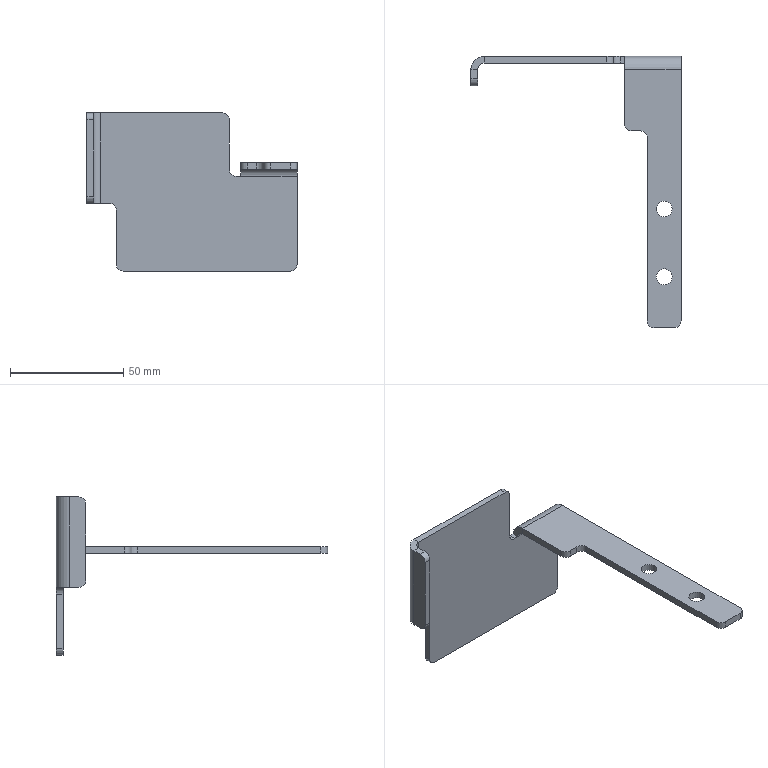Part | NX | features BREP 1 | 1 solid | 40 faces | box 93 x 120 x 70 mm | volume 23018 mm3 | plane 23 | cylinder 17 | commonest cylinder face diameters 6 x13 7 x2 12 x2
STEP:
#1=CARTESIAN_POINT('',(-17.5,-3.,-3.));
#2=VERTEX_POINT('',#1);
#3=CARTESIAN_POINT('',(-17.5,-3.,19.));
#4=VERTEX_POINT('',#3);
#5=CARTESIAN_POINT('',(-17.5,-3.,22.));
#6=DIRECTION('',(0.,0.,1.));
#7=VECTOR('',#6,1000.);
#8=LINE('',#5,#7);
#9=EDGE_CURVE('',#2,#4,#8,.T.);
#10=ORIENTED_EDGE('',*,*,#9,.T.);
#11=CARTESIAN_POINT('',(-20.5,-3.,22.));
#12=VERTEX_POINT('',#11);
#13=CARTESIAN_POINT('',(-20.5,-3.,19.));
#14=DIRECTION('',(0.,-1.,0.));
#15=DIRECTION('',(0.,0.,1.));
#16=AXIS2_PLACEMENT_3D('',#13,#14,#15);
#17=CIRCLE('',#16,3.);
#18=EDGE_CURVE('',#4,#12,#17,.T.);
#19=ORIENTED_EDGE('',*,*,#18,.T.);
#20=CARTESIAN_POINT('',(-74.5,-3.,22.));
#21=VERTEX_POINT('',#20);
#22=CARTESIAN_POINT('',(-77.5,-3.,22.));
#23=DIRECTION('',(-1.,0.,0.));
#24=VECTOR('',#23,1000.);
#25=LINE('',#22,#24);
#26=EDGE_CURVE('',#12,#21,#25,.T.);
#27=ORIENTED_EDGE('',*,*,#26,.T.);
#28=CARTESIAN_POINT('',(-74.5,-3.,-18.));
#29=VERTEX_POINT('',#28);
#30=CARTESIAN_POINT('',(-74.5,-3.,-48.));
#31=DIRECTION('',(0.,0.,1.));
#32=VECTOR('',#31,1000.);
#33=LINE('',#30,#32);
#34=EDGE_CURVE('',#29,#21,#33,.T.);
#35=ORIENTED_EDGE('',*,*,#34,.F.);
#36=CARTESIAN_POINT('',(-70.5,-3.,-18.));
#37=VERTEX_POINT('',#36);
#38=CARTESIAN_POINT('',(12.5,-3.,-18.));
#39=DIRECTION('',(1.,0.,0.));
#40=VECTOR('',#39,1000.);
#41=LINE('',#38,#40);
#42=EDGE_CURVE('',#29,#37,#41,.T.);
#43=ORIENTED_EDGE('',*,*,#42,.T.);
#44=CARTESIAN_POINT('',(-67.5,-3.,-21.));
#45=VERTEX_POINT('',#44);
#46=CARTESIAN_POINT('',(-70.5,-3.,-21.));
#47=DIRECTION('',(0.,1.,0.));
#48=DIRECTION('',(0.,0.,1.));
#49=AXIS2_PLACEMENT_3D('',#46,#47,#48);
#50=CIRCLE('',#49,3.);
#51=EDGE_CURVE('',#37,#45,#50,.T.);
#52=ORIENTED_EDGE('',*,*,#51,.T.);
#53=CARTESIAN_POINT('',(-67.5,-3.,-45.));
#54=VERTEX_POINT('',#53);
#55=CARTESIAN_POINT('',(-67.5,-3.,0.));
#56=DIRECTION('',(0.,0.,-1.));
#57=VECTOR('',#56,1000.);
#58=LINE('',#55,#57);
#59=EDGE_CURVE('',#45,#54,#58,.T.);
#60=ORIENTED_EDGE('',*,*,#59,.T.);
#61=CARTESIAN_POINT('',(-64.5,-3.,-48.));
#62=VERTEX_POINT('',#61);
#63=CARTESIAN_POINT('',(-64.5,-3.,-45.));
#64=DIRECTION('',(0.,-1.,0.));
#65=DIRECTION('',(0.,0.,1.));
#66=AXIS2_PLACEMENT_3D('',#63,#64,#65);
#67=CIRCLE('',#66,3.);
#68=EDGE_CURVE('',#54,#62,#67,.T.);
#69=ORIENTED_EDGE('',*,*,#68,.T.);
#70=CARTESIAN_POINT('',(9.5,-3.,-48.));
#71=VERTEX_POINT('',#70);
#72=CARTESIAN_POINT('',(12.5,-3.,-48.));
#73=DIRECTION('',(-1.,0.,0.));
#74=VECTOR('',#73,1000.);
#75=LINE('',#72,#74);
#76=EDGE_CURVE('',#71,#62,#75,.T.);
#77=ORIENTED_EDGE('',*,*,#76,.F.);
#78=CARTESIAN_POINT('',(12.5,-3.,-45.));
#79=VERTEX_POINT('',#78);
#80=CARTESIAN_POINT('',(9.5,-3.,-45.));
#81=DIRECTION('',(0.,-1.,0.));
#82=DIRECTION('',(0.,0.,1.));
#83=AXIS2_PLACEMENT_3D('',#80,#81,#82);
#84=CIRCLE('',#83,3.);
#85=EDGE_CURVE('',#71,#79,#84,.T.);
#86=ORIENTED_EDGE('',*,*,#85,.T.);
#87=CARTESIAN_POINT('',(12.5,-3.,-6.));
#88=VERTEX_POINT('',#87);
#89=CARTESIAN_POINT('',(12.5,-3.,0.));
#90=DIRECTION('',(0.,0.,-1.));
#91=VECTOR('',#90,1000.);
#92=LINE('',#89,#91);
#93=EDGE_CURVE('',#88,#79,#92,.T.);
#94=ORIENTED_EDGE('',*,*,#93,.F.);
#95=CARTESIAN_POINT('',(-12.5,-3.,-6.));
#96=VERTEX_POINT('',#95);
#97=CARTESIAN_POINT('',(12.5,-3.,-6.));
#98=DIRECTION('',(-1.,0.,0.));
#99=VECTOR('',#98,1000.);
#100=LINE('',#97,#99);
#101=EDGE_CURVE('',#88,#96,#100,.T.);
#102=ORIENTED_EDGE('',*,*,#101,.T.);
#103=CARTESIAN_POINT('',(-14.5,-3.,-6.));
#104=VERTEX_POINT('',#103);
#105=CARTESIAN_POINT('',(-17.5,-3.,-6.));
#106=DIRECTION('',(-1.,0.,0.));
#107=VECTOR('',#106,1000.);
#108=LINE('',#105,#107);
#109=EDGE_CURVE('',#96,#104,#108,.T.);
#110=ORIENTED_EDGE('',*,*,#109,.T.);
#111=CARTESIAN_POINT('',(-14.5,-3.,-3.));
#112=DIRECTION('',(0.,1.,0.));
#113=DIRECTION('',(0.,0.,1.));
#114=AXIS2_PLACEMENT_3D('',#111,#112,#113);
#115=CIRCLE('',#114,3.);
#116=EDGE_CURVE('',#104,#2,#115,.T.);
#117=ORIENTED_EDGE('',*,*,#116,.T.);
#118=EDGE_LOOP('',(#10,#19,#27,#35,#43,#52,#60,#69,#77,#86,#94,#102,#110,#117));
#119=FACE_BOUND('',#118,.T.);
#120=CARTESIAN_POINT('',(12.5,-3.,0.));
#121=DIRECTION('',(0.,1.,0.));
#122=DIRECTION('',(0.,0.,-1.));
#123=AXIS2_PLACEMENT_3D('',#120,#121,#122);
#124=PLANE('',#123);
#125=ADVANCED_FACE('',(#119),#124,.F.);
#126=CARTESIAN_POINT('',(9.5,0.,-48.));
#127=VERTEX_POINT('',#126);
#128=CARTESIAN_POINT('',(-64.5,0.,-48.));
#129=VERTEX_POINT('',#128);
#130=CARTESIAN_POINT('',(12.5,0.,-48.));
#131=DIRECTION('',(-1.,0.,0.));
#132=VECTOR('',#131,1000.);
#133=LINE('',#130,#132);
#134=EDGE_CURVE('',#127,#129,#133,.T.);
#135=ORIENTED_EDGE('',*,*,#134,.F.);
#136=CARTESIAN_POINT('',(9.5,0.,-48.));
#137=DIRECTION('',(0.,-1.,0.));
#138=VECTOR('',#137,1000.);
#139=LINE('',#136,#138);
#140=EDGE_CURVE('',#127,#71,#139,.T.);
#141=ORIENTED_EDGE('',*,*,#140,.T.);
#142=ORIENTED_EDGE('',*,*,#76,.T.);
#143=CARTESIAN_POINT('',(-64.5,0.,-48.));
#144=DIRECTION('',(0.,1.,0.));
#145=VECTOR('',#144,1000.);
#146=LINE('',#143,#145);
#147=EDGE_CURVE('',#62,#129,#146,.T.);
#148=ORIENTED_EDGE('',*,*,#147,.T.);
#149=EDGE_LOOP('',(#135,#141,#142,#148));
#150=FACE_BOUND('',#149,.T.);
#151=CARTESIAN_POINT('',(12.5,0.,-48.));
#152=DIRECTION('',(0.,0.,-1.));
#153=DIRECTION('',(1.,0.,0.));
#154=AXIS2_PLACEMENT_3D('',#151,#152,#153);
#155=PLANE('',#154);
#156=ADVANCED_FACE('',(#150),#155,.T.);
#157=CARTESIAN_POINT('',(-74.5,0.,22.));
#158=VERTEX_POINT('',#157);
#159=CARTESIAN_POINT('',(-20.5,0.,22.));
#160=VERTEX_POINT('',#159);
#161=CARTESIAN_POINT('',(-77.5,0.,22.));
#162=DIRECTION('',(1.,0.,0.));
#163=VECTOR('',#162,1000.);
#164=LINE('',#161,#163);
#165=EDGE_CURVE('',#158,#160,#164,.T.);
#166=ORIENTED_EDGE('',*,*,#165,.T.);
#167=CARTESIAN_POINT('',(-17.5,0.,19.));
#168=VERTEX_POINT('',#167);
#169=CARTESIAN_POINT('',(-20.5,0.,19.));
#170=DIRECTION('',(0.,1.,0.));
#171=DIRECTION('',(0.,0.,1.));
#172=AXIS2_PLACEMENT_3D('',#169,#170,#171);
#173=CIRCLE('',#172,3.);
#174=EDGE_CURVE('',#160,#168,#173,.T.);
#175=ORIENTED_EDGE('',*,*,#174,.T.);
#176=CARTESIAN_POINT('',(-17.5,0.,-3.));
#177=VERTEX_POINT('',#176);
#178=CARTESIAN_POINT('',(-17.5,0.,22.));
#179=DIRECTION('',(0.,0.,-1.));
#180=VECTOR('',#179,1000.);
#181=LINE('',#178,#180);
#182=EDGE_CURVE('',#168,#177,#181,.T.);
#183=ORIENTED_EDGE('',*,*,#182,.T.);
#184=CARTESIAN_POINT('',(-14.5,0.,-6.));
#185=VERTEX_POINT('',#184);
#186=CARTESIAN_POINT('',(-14.5,0.,-3.));
#187=DIRECTION('',(0.,-1.,0.));
#188=DIRECTION('',(0.,0.,1.));
#189=AXIS2_PLACEMENT_3D('',#186,#187,#188);
#190=CIRCLE('',#189,3.);
#191=EDGE_CURVE('',#177,#185,#190,.T.);
#192=ORIENTED_EDGE('',*,*,#191,.T.);
#193=CARTESIAN_POINT('',(-12.5,0.,-6.));
#194=VERTEX_POINT('',#193);
#195=CARTESIAN_POINT('',(-17.5,0.,-6.));
#196=DIRECTION('',(1.,0.,0.));
#197=VECTOR('',#196,1000.);
#198=LINE('',#195,#197);
#199=EDGE_CURVE('',#185,#194,#198,.T.);
#200=ORIENTED_EDGE('',*,*,#199,.T.);
#201=CARTESIAN_POINT('',(12.5,0.,-6.));
#202=VERTEX_POINT('',#201);
#203=CARTESIAN_POINT('',(12.5,0.,-6.));
#204=DIRECTION('',(-1.,0.,0.));
#205=VECTOR('',#204,1000.);
#206=LINE('',#203,#205);
#207=EDGE_CURVE('',#202,#194,#206,.T.);
#208=ORIENTED_EDGE('',*,*,#207,.F.);
#209=CARTESIAN_POINT('',(12.5,0.,-45.));
#210=VERTEX_POINT('',#209);
#211=CARTESIAN_POINT('',(12.5,0.,0.));
#212=DIRECTION('',(0.,0.,-1.));
#213=VECTOR('',#212,1000.);
#214=LINE('',#211,#213);
#215=EDGE_CURVE('',#202,#210,#214,.T.);
#216=ORIENTED_EDGE('',*,*,#215,.T.);
#217=CARTESIAN_POINT('',(9.5,0.,-45.));
#218=DIRECTION('',(0.,1.,0.));
#219=DIRECTION('',(0.,0.,1.));
#220=AXIS2_PLACEMENT_3D('',#217,#218,#219);
#221=CIRCLE('',#220,3.);
#222=EDGE_CURVE('',#210,#127,#221,.T.);
#223=ORIENTED_EDGE('',*,*,#222,.T.);
#224=ORIENTED_EDGE('',*,*,#134,.T.);
#225=CARTESIAN_POINT('',(-67.5,0.,-45.));
#226=VERTEX_POINT('',#225);
#227=CARTESIAN_POINT('',(-64.5,0.,-45.));
#228=DIRECTION('',(0.,1.,0.));
#229=DIRECTION('',(0.,0.,1.));
#230=AXIS2_PLACEMENT_3D('',#227,#228,#229);
#231=CIRCLE('',#230,3.);
#232=EDGE_CURVE('',#129,#226,#231,.T.);
#233=ORIENTED_EDGE('',*,*,#232,.T.);
#234=CARTESIAN_POINT('',(-67.5,0.,-21.));
#235=VERTEX_POINT('',#234);
#236=CARTESIAN_POINT('',(-67.5,0.,-48.));
#237=DIRECTION('',(0.,0.,-1.));
#238=VECTOR('',#237,1000.);
#239=LINE('',#236,#238);
#240=EDGE_CURVE('',#235,#226,#239,.T.);
#241=ORIENTED_EDGE('',*,*,#240,.F.);
#242=CARTESIAN_POINT('',(-70.5,0.,-18.));
#243=VERTEX_POINT('',#242);
#244=CARTESIAN_POINT('',(-70.5,0.,-21.));
#245=DIRECTION('',(0.,-1.,0.));
#246=DIRECTION('',(0.,0.,1.));
#247=AXIS2_PLACEMENT_3D('',#244,#245,#246);
#248=CIRCLE('',#247,3.);
#249=EDGE_CURVE('',#235,#243,#248,.T.);
#250=ORIENTED_EDGE('',*,*,#249,.T.);
#251=CARTESIAN_POINT('',(-74.5,0.,-18.));
#252=VERTEX_POINT('',#251);
#253=CARTESIAN_POINT('',(-67.5,0.,-18.));
#254=DIRECTION('',(1.,0.,0.));
#255=VECTOR('',#254,1000.);
#256=LINE('',#253,#255);
#257=EDGE_CURVE('',#252,#243,#256,.T.);
#258=ORIENTED_EDGE('',*,*,#257,.F.);
#259=CARTESIAN_POINT('',(-74.5,0.,-48.));
#260=DIRECTION('',(0.,0.,1.));
#261=VECTOR('',#260,1000.);
#262=LINE('',#259,#261);
#263=EDGE_CURVE('',#252,#158,#262,.T.);
#264=ORIENTED_EDGE('',*,*,#263,.T.);
#265=EDGE_LOOP('',(#166,#175,#183,#192,#200,#208,#216,#223,#224,#233,#241,#250,#258,#264));
#266=FACE_BOUND('',#265,.T.);
#267=CARTESIAN_POINT('',(12.5,0.,0.));
#268=DIRECTION('',(0.,1.,0.));
#269=DIRECTION('',(0.,0.,-1.));
#270=AXIS2_PLACEMENT_3D('',#267,#268,#269);
#271=PLANE('',#270);
#272=ADVANCED_FACE('',(#266),#271,.T.);
#273=CARTESIAN_POINT('',(12.5,0.,-6.));
#274=DIRECTION('',(0.,-1.,0.));
#275=VECTOR('',#274,1000.);
#276=LINE('',#273,#275);
#277=EDGE_CURVE('',#202,#88,#276,.T.);
#278=ORIENTED_EDGE('',*,*,#277,.F.);
#279=CARTESIAN_POINT('',(12.5,-6.,0.));
#280=VERTEX_POINT('',#279);
#281=CARTESIAN_POINT('',(12.5,-6.,-6.));
#282=DIRECTION('',(-1.,0.,0.));
#283=DIRECTION('',(0.,0.,-1.));
#284=AXIS2_PLACEMENT_3D('',#281,#282,#283);
#285=CIRCLE('',#284,6.);
#286=EDGE_CURVE('',#280,#202,#285,.T.);
#287=ORIENTED_EDGE('',*,*,#286,.F.);
#288=CARTESIAN_POINT('',(12.5,-6.,-3.));
#289=VERTEX_POINT('',#288);
#290=CARTESIAN_POINT('',(12.5,-6.,-3.));
#291=DIRECTION('',(0.,0.,1.));
#292=VECTOR('',#291,1000.);
#293=LINE('',#290,#292);
#294=EDGE_CURVE('',#289,#280,#293,.T.);
#295=ORIENTED_EDGE('',*,*,#294,.F.);
#296=CARTESIAN_POINT('',(12.5,-6.,-6.));
#297=DIRECTION('',(-1.,0.,0.));
#298=DIRECTION('',(0.,0.,-1.));
#299=AXIS2_PLACEMENT_3D('',#296,#297,#298);
#300=CIRCLE('',#299,3.);
#301=EDGE_CURVE('',#289,#88,#300,.T.);
#302=ORIENTED_EDGE('',*,*,#301,.T.);
#303=EDGE_LOOP('',(#278,#287,#295,#302));
#304=FACE_BOUND('',#303,.T.);
#305=CARTESIAN_POINT('',(12.5,0.,-6.));
#306=DIRECTION('',(1.,0.,0.));
#307=DIRECTION('',(0.,0.,1.));
#308=AXIS2_PLACEMENT_3D('',#305,#306,#307);
#309=PLANE('',#308);
#310=ADVANCED_FACE('',(#304),#309,.T.);
#311=ORIENTED_EDGE('',*,*,#93,.T.);
#312=CARTESIAN_POINT('',(12.5,-6.,-45.));
#313=DIRECTION('',(0.,1.,0.));
#314=VECTOR('',#313,1000.);
#315=LINE('',#312,#314);
#316=EDGE_CURVE('',#79,#210,#315,.T.);
#317=ORIENTED_EDGE('',*,*,#316,.T.);
#318=ORIENTED_EDGE('',*,*,#215,.F.);
#319=ORIENTED_EDGE('',*,*,#277,.T.);
#320=EDGE_LOOP('',(#311,#317,#318,#319));
#321=FACE_BOUND('',#320,.T.);
#322=CARTESIAN_POINT('',(12.5,-6.,-3.));
#323=DIRECTION('',(1.,0.,0.));
#324=DIRECTION('',(0.,0.,1.));
#325=AXIS2_PLACEMENT_3D('',#322,#323,#324);
#326=PLANE('',#325);
#327=ADVANCED_FACE('',(#321),#326,.T.);
#328=CARTESIAN_POINT('',(-12.5,-6.,0.));
#329=VERTEX_POINT('',#328);
#330=CARTESIAN_POINT('',(-12.5,-6.,-3.));
#331=VERTEX_POINT('',#330);
#332=CARTESIAN_POINT('',(-12.5,-6.,0.));
#333=DIRECTION('',(0.,0.,-1.));
#334=VECTOR('',#333,1000.);
#335=LINE('',#332,#334);
#336=EDGE_CURVE('',#329,#331,#335,.T.);
#337=ORIENTED_EDGE('',*,*,#336,.F.);
#338=CARTESIAN_POINT('',(-12.5,-6.,-6.));
#339=DIRECTION('',(-1.,0.,0.));
#340=DIRECTION('',(0.,0.,-1.));
#341=AXIS2_PLACEMENT_3D('',#338,#339,#340);
#342=CIRCLE('',#341,6.);
#343=EDGE_CURVE('',#329,#194,#342,.T.);
#344=ORIENTED_EDGE('',*,*,#343,.T.);
#345=CARTESIAN_POINT('',(-12.5,-3.,-6.));
#346=DIRECTION('',(0.,1.,0.));
#347=VECTOR('',#346,1000.);
#348=LINE('',#345,#347);
#349=EDGE_CURVE('',#96,#194,#348,.T.);
#350=ORIENTED_EDGE('',*,*,#349,.F.);
#351=CARTESIAN_POINT('',(-12.5,-6.,-6.));
#352=DIRECTION('',(-1.,0.,0.));
#353=DIRECTION('',(0.,0.,-1.));
#354=AXIS2_PLACEMENT_3D('',#351,#352,#353);
#355=CIRCLE('',#354,3.);
#356=EDGE_CURVE('',#331,#96,#355,.T.);
#357=ORIENTED_EDGE('',*,*,#356,.F.);
#358=EDGE_LOOP('',(#337,#344,#350,#357));
#359=FACE_BOUND('',#358,.T.);
#360=CARTESIAN_POINT('',(-12.5,-6.,0.));
#361=DIRECTION('',(-1.,0.,0.));
#362=DIRECTION('',(0.,0.,-1.));
#363=AXIS2_PLACEMENT_3D('',#360,#361,#362);
#364=PLANE('',#363);
#365=ADVANCED_FACE('',(#359),#364,.T.);
#366=CARTESIAN_POINT('',(-12.5,-30.,-3.));
#367=VERTEX_POINT('',#366);
#368=CARTESIAN_POINT('',(-12.5,-120.,-3.));
#369=DIRECTION('',(0.,1.,0.));
#370=VECTOR('',#369,1000.);
#371=LINE('',#368,#370);
#372=EDGE_CURVE('',#367,#331,#371,.T.);
#373=ORIENTED_EDGE('',*,*,#372,.F.);
#374=CARTESIAN_POINT('',(-12.5,-30.,0.));
#375=VERTEX_POINT('',#374);
#376=CARTESIAN_POINT('',(-12.5,-30.,0.));
#377=DIRECTION('',(0.,0.,1.));
#378=VECTOR('',#377,1000.);
#379=LINE('',#376,#378);
#380=EDGE_CURVE('',#367,#375,#379,.T.);
#381=ORIENTED_EDGE('',*,*,#380,.T.);
#382=CARTESIAN_POINT('',(-12.5,-120.,0.));
#383=DIRECTION('',(0.,1.,0.));
#384=VECTOR('',#383,1000.);
#385=LINE('',#382,#384);
#386=EDGE_CURVE('',#375,#329,#385,.T.);
#387=ORIENTED_EDGE('',*,*,#386,.T.);
#388=ORIENTED_EDGE('',*,*,#336,.T.);
#389=EDGE_LOOP('',(#373,#381,#387,#388));
#390=FACE_BOUND('',#389,.T.);
#391=CARTESIAN_POINT('',(-12.5,-3.,-6.));
#392=DIRECTION('',(-1.,0.,0.));
#393=DIRECTION('',(0.,0.,-1.));
#394=AXIS2_PLACEMENT_3D('',#391,#392,#393);
#395=PLANE('',#394);
#396=ADVANCED_FACE('',(#390),#395,.T.);
#397=ORIENTED_EDGE('',*,*,#343,.F.);
#398=CARTESIAN_POINT('',(12.5,-6.,0.));
#399=DIRECTION('',(-1.,0.,0.));
#400=VECTOR('',#399,1000.);
#401=LINE('',#398,#400);
#402=EDGE_CURVE('',#280,#329,#401,.T.);
#403=ORIENTED_EDGE('',*,*,#402,.F.);
#404=ORIENTED_EDGE('',*,*,#286,.T.);
#405=ORIENTED_EDGE('',*,*,#207,.T.);
#406=EDGE_LOOP('',(#397,#403,#404,#405));
#407=FACE_BOUND('',#406,.T.);
#408=CARTESIAN_POINT('',(12.5,-6.,-6.));
#409=DIRECTION('',(-1.,0.,0.));
#410=DIRECTION('',(0.,0.,-1.));
#411=AXIS2_PLACEMENT_3D('',#408,#409,#410);
#412=CYLINDRICAL_SURFACE('',#411,6.);
#413=ADVANCED_FACE('',(#407),#412,.T.);
#414=CARTESIAN_POINT('',(8.5,-67.5,0.));
#415=VERTEX_POINT('',#414);
#416=CARTESIAN_POINT('',(5.,-67.5,0.));
#417=DIRECTION('',(0.,0.,1.));
#418=DIRECTION('',(1.,0.,0.));
#419=AXIS2_PLACEMENT_3D('',#416,#417,#418);
#420=CIRCLE('',#419,3.5);
#421=EDGE_CURVE('',#415,#415,#420,.T.);
#422=ORIENTED_EDGE('',*,*,#421,.F.);
#423=EDGE_LOOP('',(#422));
#424=FACE_BOUND('',#423,.T.);
#425=CARTESIAN_POINT('',(8.5,-97.5,0.));
#426=VERTEX_POINT('',#425);
#427=CARTESIAN_POINT('',(5.,-97.5,0.));
#428=DIRECTION('',(0.,0.,1.));
#429=DIRECTION('',(1.,0.,0.));
#430=AXIS2_PLACEMENT_3D('',#427,#428,#429);
#431=CIRCLE('',#430,3.5);
#432=EDGE_CURVE('',#426,#426,#431,.T.);
#433=ORIENTED_EDGE('',*,*,#432,.F.);
#434=EDGE_LOOP('',(#433));
#435=FACE_BOUND('',#434,.T.);
#436=CARTESIAN_POINT('',(9.5,-120.,0.));
#437=VERTEX_POINT('',#436);
#438=CARTESIAN_POINT('',(0.5,-120.,0.));
#439=VERTEX_POINT('',#438);
#440=CARTESIAN_POINT('',(12.5,-120.,0.));
#441=DIRECTION('',(-1.,0.,0.));
#442=VECTOR('',#441,1000.);
#443=LINE('',#440,#442);
#444=EDGE_CURVE('',#437,#439,#443,.T.);
#445=ORIENTED_EDGE('',*,*,#444,.F.);
#446=CARTESIAN_POINT('',(12.5,-117.,0.));
#447=VERTEX_POINT('',#446);
#448=CARTESIAN_POINT('',(9.5,-117.,0.));
#449=DIRECTION('',(0.,0.,1.));
#450=DIRECTION('',(1.,0.,0.));
#451=AXIS2_PLACEMENT_3D('',#448,#449,#450);
#452=CIRCLE('',#451,3.);
#453=EDGE_CURVE('',#437,#447,#452,.T.);
#454=ORIENTED_EDGE('',*,*,#453,.T.);
#455=CARTESIAN_POINT('',(12.5,-120.,0.));
#456=DIRECTION('',(0.,1.,0.));
#457=VECTOR('',#456,1000.);
#458=LINE('',#455,#457);
#459=EDGE_CURVE('',#447,#280,#458,.T.);
#460=ORIENTED_EDGE('',*,*,#459,.T.);
#461=ORIENTED_EDGE('',*,*,#402,.T.);
#462=ORIENTED_EDGE('',*,*,#386,.F.);
#463=CARTESIAN_POINT('',(-9.5,-33.,0.));
#464=VERTEX_POINT('',#463);
#465=CARTESIAN_POINT('',(-9.5,-30.,0.));
#466=DIRECTION('',(0.,0.,1.));
#467=DIRECTION('',(1.,0.,0.));
#468=AXIS2_PLACEMENT_3D('',#465,#466,#467);
#469=CIRCLE('',#468,3.);
#470=EDGE_CURVE('',#375,#464,#469,.T.);
#471=ORIENTED_EDGE('',*,*,#470,.T.);
#472=CARTESIAN_POINT('',(-5.5,-33.,0.));
#473=VERTEX_POINT('',#472);
#474=CARTESIAN_POINT('',(-12.5,-33.,0.));
#475=DIRECTION('',(-1.,0.,0.));
#476=VECTOR('',#475,1000.);
#477=LINE('',#474,#476);
#478=EDGE_CURVE('',#473,#464,#477,.T.);
#479=ORIENTED_EDGE('',*,*,#478,.F.);
#480=CARTESIAN_POINT('',(-2.5,-36.,0.));
#481=VERTEX_POINT('',#480);
#482=CARTESIAN_POINT('',(-5.5,-36.,0.));
#483=DIRECTION('',(0.,0.,-1.));
#484=DIRECTION('',(1.,0.,0.));
#485=AXIS2_PLACEMENT_3D('',#482,#483,#484);
#486=CIRCLE('',#485,3.);
#487=EDGE_CURVE('',#473,#481,#486,.T.);
#488=ORIENTED_EDGE('',*,*,#487,.T.);
#489=CARTESIAN_POINT('',(-2.5,-117.,0.));
#490=VERTEX_POINT('',#489);
#491=CARTESIAN_POINT('',(-2.5,-120.,0.));
#492=DIRECTION('',(0.,1.,0.));
#493=VECTOR('',#492,1000.);
#494=LINE('',#491,#493);
#495=EDGE_CURVE('',#490,#481,#494,.T.);
#496=ORIENTED_EDGE('',*,*,#495,.F.);
#497=CARTESIAN_POINT('',(0.5,-117.,0.));
#498=DIRECTION('',(0.,0.,1.));
#499=DIRECTION('',(1.,0.,0.));
#500=AXIS2_PLACEMENT_3D('',#497,#498,#499);
#501=CIRCLE('',#500,3.);
#502=EDGE_CURVE('',#490,#439,#501,.T.);
#503=ORIENTED_EDGE('',*,*,#502,.T.);
#504=EDGE_LOOP('',(#445,#454,#460,#461,#462,#471,#479,#488,#496,#503));
#505=FACE_BOUND('',#504,.T.);
#506=CARTESIAN_POINT('',(12.5,-120.,0.));
#507=DIRECTION('',(0.,0.,1.));
#508=DIRECTION('',(-1.,0.,0.));
#509=AXIS2_PLACEMENT_3D('',#506,#507,#508);
#510=PLANE('',#509);
#511=ADVANCED_FACE('',(#424,#435,#505),#510,.T.);
#512=CARTESIAN_POINT('',(9.5,-120.,-3.));
#513=VERTEX_POINT('',#512);
#514=CARTESIAN_POINT('',(0.5,-120.,-3.));
#515=VERTEX_POINT('',#514);
#516=CARTESIAN_POINT('',(12.5,-120.,-3.));
#517=DIRECTION('',(-1.,0.,0.));
#518=VECTOR('',#517,1000.);
#519=LINE('',#516,#518);
#520=EDGE_CURVE('',#513,#515,#519,.T.);
#521=ORIENTED_EDGE('',*,*,#520,.F.);
#522=CARTESIAN_POINT('',(9.5,-120.,-3.));
#523=DIRECTION('',(0.,0.,1.));
#524=VECTOR('',#523,1000.);
#525=LINE('',#522,#524);
#526=EDGE_CURVE('',#513,#437,#525,.T.);
#527=ORIENTED_EDGE('',*,*,#526,.T.);
#528=ORIENTED_EDGE('',*,*,#444,.T.);
#529=CARTESIAN_POINT('',(0.5,-120.,-3.));
#530=DIRECTION('',(0.,0.,-1.));
#531=VECTOR('',#530,1000.);
#532=LINE('',#529,#531);
#533=EDGE_CURVE('',#439,#515,#532,.T.);
#534=ORIENTED_EDGE('',*,*,#533,.T.);
#535=EDGE_LOOP('',(#521,#527,#528,#534));
#536=FACE_BOUND('',#535,.T.);
#537=CARTESIAN_POINT('',(12.5,-120.,-3.));
#538=DIRECTION('',(0.,-1.,0.));
#539=DIRECTION('',(0.,0.,1.));
#540=AXIS2_PLACEMENT_3D('',#537,#538,#539);
#541=PLANE('',#540);
#542=ADVANCED_FACE('',(#536),#541,.T.);
#543=CARTESIAN_POINT('',(8.5,-67.5,-3.));
#544=VERTEX_POINT('',#543);
#545=CARTESIAN_POINT('',(5.,-67.5,-3.));
#546=DIRECTION('',(0.,0.,1.));
#547=DIRECTION('',(1.,0.,0.));
#548=AXIS2_PLACEMENT_3D('',#545,#546,#547);
#549=CIRCLE('',#548,3.5);
#550=EDGE_CURVE('',#544,#544,#549,.T.);
#551=ORIENTED_EDGE('',*,*,#550,.T.);
#552=EDGE_LOOP('',(#551));
#553=FACE_BOUND('',#552,.T.);
#554=CARTESIAN_POINT('',(8.5,-97.5,-3.));
#555=VERTEX_POINT('',#554);
#556=CARTESIAN_POINT('',(5.,-97.5,-3.));
#557=DIRECTION('',(0.,0.,1.));
#558=DIRECTION('',(1.,0.,0.));
#559=AXIS2_PLACEMENT_3D('',#556,#557,#558);
#560=CIRCLE('',#559,3.5);
#561=EDGE_CURVE('',#555,#555,#560,.T.);
#562=ORIENTED_EDGE('',*,*,#561,.T.);
#563=EDGE_LOOP('',(#562));
#564=FACE_BOUND('',#563,.T.);
#565=CARTESIAN_POINT('',(12.5,-117.,-3.));
#566=VERTEX_POINT('',#565);
#567=CARTESIAN_POINT('',(12.5,-120.,-3.));
#568=DIRECTION('',(0.,1.,0.));
#569=VECTOR('',#568,1000.);
#570=LINE('',#567,#569);
#571=EDGE_CURVE('',#566,#289,#570,.T.);
#572=ORIENTED_EDGE('',*,*,#571,.F.);
#573=CARTESIAN_POINT('',(9.5,-117.,-3.));
#574=DIRECTION('',(0.,0.,-1.));
#575=DIRECTION('',(1.,0.,0.));
#576=AXIS2_PLACEMENT_3D('',#573,#574,#575);
#577=CIRCLE('',#576,3.);
#578=EDGE_CURVE('',#566,#513,#577,.T.);
#579=ORIENTED_EDGE('',*,*,#578,.T.);
#580=ORIENTED_EDGE('',*,*,#520,.T.);
#581=CARTESIAN_POINT('',(-2.5,-117.,-3.));
#582=VERTEX_POINT('',#581);
#583=CARTESIAN_POINT('',(0.5,-117.,-3.));
#584=DIRECTION('',(0.,0.,-1.));
#585=DIRECTION('',(1.,0.,0.));
#586=AXIS2_PLACEMENT_3D('',#583,#584,#585);
#587=CIRCLE('',#586,3.);
#588=EDGE_CURVE('',#515,#582,#587,.T.);
#589=ORIENTED_EDGE('',*,*,#588,.T.);
#590=CARTESIAN_POINT('',(-2.5,-36.,-3.));
#591=VERTEX_POINT('',#590);
#592=CARTESIAN_POINT('',(-2.5,-120.,-3.));
#593=DIRECTION('',(0.,-1.,0.));
#594=VECTOR('',#593,1000.);
#595=LINE('',#592,#594);
#596=EDGE_CURVE('',#591,#582,#595,.T.);
#597=ORIENTED_EDGE('',*,*,#596,.F.);
#598=CARTESIAN_POINT('',(-5.5,-33.,-3.));
#599=VERTEX_POINT('',#598);
#600=CARTESIAN_POINT('',(-5.5,-36.,-3.));
#601=DIRECTION('',(0.,0.,1.));
#602=DIRECTION('',(1.,0.,0.));
#603=AXIS2_PLACEMENT_3D('',#600,#601,#602);
#604=CIRCLE('',#603,3.);
#605=EDGE_CURVE('',#591,#599,#604,.T.);
#606=ORIENTED_EDGE('',*,*,#605,.T.);
#607=CARTESIAN_POINT('',(-9.5,-33.,-3.));
#608=VERTEX_POINT('',#607);
#609=CARTESIAN_POINT('',(-12.5,-33.,-3.));
#610=DIRECTION('',(1.,0.,0.));
#611=VECTOR('',#610,1000.);
#612=LINE('',#609,#611);
#613=EDGE_CURVE('',#608,#599,#612,.T.);
#614=ORIENTED_EDGE('',*,*,#613,.F.);
#615=CARTESIAN_POINT('',(-9.5,-30.,-3.));
#616=DIRECTION('',(0.,0.,-1.));
#617=DIRECTION('',(1.,0.,0.));
#618=AXIS2_PLACEMENT_3D('',#615,#616,#617);
#619=CIRCLE('',#618,3.);
#620=EDGE_CURVE('',#608,#367,#619,.T.);
#621=ORIENTED_EDGE('',*,*,#620,.T.);
#622=ORIENTED_EDGE('',*,*,#372,.T.);
#623=CARTESIAN_POINT('',(12.5,-6.,-3.));
#624=DIRECTION('',(-1.,0.,0.));
#625=VECTOR('',#624,1000.);
#626=LINE('',#623,#625);
#627=EDGE_CURVE('',#289,#331,#626,.T.);
#628=ORIENTED_EDGE('',*,*,#627,.F.);
#629=EDGE_LOOP('',(#572,#579,#580,#589,#597,#606,#614,#621,#622,#628));
#630=FACE_BOUND('',#629,.T.);
#631=CARTESIAN_POINT('',(12.5,-120.,-3.));
#632=DIRECTION('',(0.,0.,1.));
#633=DIRECTION('',(-1.,0.,0.));
#634=AXIS2_PLACEMENT_3D('',#631,#632,#633);
#635=PLANE('',#634);
#636=ADVANCED_FACE('',(#553,#564,#630),#635,.F.);
#637=ORIENTED_EDGE('',*,*,#356,.T.);
#638=ORIENTED_EDGE('',*,*,#101,.F.);
#639=ORIENTED_EDGE('',*,*,#301,.F.);
#640=ORIENTED_EDGE('',*,*,#627,.T.);
#641=EDGE_LOOP('',(#637,#638,#639,#640));
#642=FACE_BOUND('',#641,.T.);
#643=CARTESIAN_POINT('',(12.5,-6.,-6.));
#644=DIRECTION('',(-1.,0.,0.));
#645=DIRECTION('',(0.,0.,-1.));
#646=AXIS2_PLACEMENT_3D('',#643,#644,#645);
#647=CYLINDRICAL_SURFACE('',#646,3.);
#648=ADVANCED_FACE('',(#642),#647,.F.);
#649=ORIENTED_EDGE('',*,*,#459,.F.);
#650=CARTESIAN_POINT('',(12.5,-117.,-6.));
#651=DIRECTION('',(0.,0.,-1.));
#652=VECTOR('',#651,1000.);
#653=LINE('',#650,#652);
#654=EDGE_CURVE('',#447,#566,#653,.T.);
#655=ORIENTED_EDGE('',*,*,#654,.T.);
#656=ORIENTED_EDGE('',*,*,#571,.T.);
#657=ORIENTED_EDGE('',*,*,#294,.T.);
#658=EDGE_LOOP('',(#649,#655,#656,#657));
#659=FACE_BOUND('',#658,.T.);
#660=CARTESIAN_POINT('',(12.5,-6.,-6.));
#661=DIRECTION('',(1.,0.,0.));
#662=DIRECTION('',(0.,0.,1.));
#663=AXIS2_PLACEMENT_3D('',#660,#661,#662);
#664=PLANE('',#663);
#665=ADVANCED_FACE('',(#659),#664,.T.);
#666=ORIENTED_EDGE('',*,*,#199,.F.);
#667=CARTESIAN_POINT('',(-14.5,-3.,-6.));
#668=DIRECTION('',(0.,-1.,0.));
#669=VECTOR('',#668,1000.);
#670=LINE('',#667,#669);
#671=EDGE_CURVE('',#185,#104,#670,.T.);
#672=ORIENTED_EDGE('',*,*,#671,.T.);
#673=ORIENTED_EDGE('',*,*,#109,.F.);
#674=ORIENTED_EDGE('',*,*,#349,.T.);
#675=EDGE_LOOP('',(#666,#672,#673,#674));
#676=FACE_BOUND('',#675,.T.);
#677=CARTESIAN_POINT('',(-17.5,-98.525,-6.));
#678=DIRECTION('',(0.,0.,1.));
#679=DIRECTION('',(-1.,0.,0.));
#680=AXIS2_PLACEMENT_3D('',#677,#678,#679);
#681=PLANE('',#680);
#682=ADVANCED_FACE('',(#676),#681,.T.);
#683=ORIENTED_EDGE('',*,*,#9,.F.);
#684=CARTESIAN_POINT('',(-17.5,0.,-3.));
#685=DIRECTION('',(0.,1.,0.));
#686=VECTOR('',#685,1000.);
#687=LINE('',#684,#686);
#688=EDGE_CURVE('',#2,#177,#687,.T.);
#689=ORIENTED_EDGE('',*,*,#688,.T.);
#690=ORIENTED_EDGE('',*,*,#182,.F.);
#691=CARTESIAN_POINT('',(-17.5,-98.525,19.));
#692=DIRECTION('',(0.,-1.,0.));
#693=VECTOR('',#692,1000.);
#694=LINE('',#691,#693);
#695=EDGE_CURVE('',#168,#4,#694,.T.);
#696=ORIENTED_EDGE('',*,*,#695,.T.);
#697=EDGE_LOOP('',(#683,#689,#690,#696));
#698=FACE_BOUND('',#697,.T.);
#699=CARTESIAN_POINT('',(-17.5,-98.525,22.));
#700=DIRECTION('',(1.,0.,0.));
#701=DIRECTION('',(0.,0.,1.));
#702=AXIS2_PLACEMENT_3D('',#699,#700,#701);
#703=PLANE('',#702);
#704=ADVANCED_FACE('',(#698),#703,.T.);
#705=ORIENTED_EDGE('',*,*,#26,.F.);
#706=CARTESIAN_POINT('',(-20.5,-98.525,22.));
#707=DIRECTION('',(0.,1.,0.));
#708=VECTOR('',#707,1000.);
#709=LINE('',#706,#708);
#710=EDGE_CURVE('',#12,#160,#709,.T.);
#711=ORIENTED_EDGE('',*,*,#710,.T.);
#712=ORIENTED_EDGE('',*,*,#165,.F.);
#713=CARTESIAN_POINT('',(-74.5,-3.,22.));
#714=DIRECTION('',(0.,1.,0.));
#715=VECTOR('',#714,1000.);
#716=LINE('',#713,#715);
#717=EDGE_CURVE('',#21,#158,#716,.T.);
#718=ORIENTED_EDGE('',*,*,#717,.F.);
#719=EDGE_LOOP('',(#705,#711,#712,#718));
#720=FACE_BOUND('',#719,.T.);
#721=CARTESIAN_POINT('',(-77.5,-98.525,22.));
#722=DIRECTION('',(0.,0.,1.));
#723=DIRECTION('',(-1.,0.,0.));
#724=AXIS2_PLACEMENT_3D('',#721,#722,#723);
#725=PLANE('',#724);
#726=ADVANCED_FACE('',(#720),#725,.T.);
#727=CARTESIAN_POINT('',(-77.5,-6.,22.));
#728=VERTEX_POINT('',#727);
#729=CARTESIAN_POINT('',(-80.5,-6.,22.));
#730=VERTEX_POINT('',#729);
#731=CARTESIAN_POINT('',(-77.5,-6.,22.));
#732=DIRECTION('',(-1.,0.,0.));
#733=VECTOR('',#732,1000.);
#734=LINE('',#731,#733);
#735=EDGE_CURVE('',#728,#730,#734,.T.);
#736=ORIENTED_EDGE('',*,*,#735,.F.);
#737=CARTESIAN_POINT('',(-74.5,-6.,22.));
#738=DIRECTION('',(0.,0.,1.));
#739=DIRECTION('',(-1.,0.,0.));
#740=AXIS2_PLACEMENT_3D('',#737,#738,#739);
#741=CIRCLE('',#740,3.);
#742=EDGE_CURVE('',#21,#728,#741,.T.);
#743=ORIENTED_EDGE('',*,*,#742,.F.);
#744=ORIENTED_EDGE('',*,*,#717,.T.);
#745=CARTESIAN_POINT('',(-74.5,-6.,22.));
#746=DIRECTION('',(0.,0.,1.));
#747=DIRECTION('',(-1.,0.,0.));
#748=AXIS2_PLACEMENT_3D('',#745,#746,#747);
#749=CIRCLE('',#748,6.);
#750=EDGE_CURVE('',#158,#730,#749,.T.);
#751=ORIENTED_EDGE('',*,*,#750,.T.);
#752=EDGE_LOOP('',(#736,#743,#744,#751));
#753=FACE_BOUND('',#752,.T.);
#754=CARTESIAN_POINT('',(-74.5,-6.,22.));
#755=DIRECTION('',(0.,0.,1.));
#756=DIRECTION('',(-1.,0.,0.));
#757=AXIS2_PLACEMENT_3D('',#754,#755,#756);
#758=PLANE('',#757);
#759=ADVANCED_FACE('',(#753),#758,.T.);
#760=CARTESIAN_POINT('',(-80.5,-6.,-18.));
#761=VERTEX_POINT('',#760);
#762=CARTESIAN_POINT('',(-74.5,-6.,-18.));
#763=DIRECTION('',(0.,0.,-1.));
#764=DIRECTION('',(1.,0.,0.));
#765=AXIS2_PLACEMENT_3D('',#762,#763,#764);
#766=CIRCLE('',#765,6.);
#767=EDGE_CURVE('',#761,#252,#766,.T.);
#768=ORIENTED_EDGE('',*,*,#767,.F.);
#769=CARTESIAN_POINT('',(-80.5,-6.,0.));
#770=DIRECTION('',(0.,0.,1.));
#771=VECTOR('',#770,1000.);
#772=LINE('',#769,#771);
#773=EDGE_CURVE('',#761,#730,#772,.T.);
#774=ORIENTED_EDGE('',*,*,#773,.T.);
#775=ORIENTED_EDGE('',*,*,#750,.F.);
#776=ORIENTED_EDGE('',*,*,#263,.F.);
#777=EDGE_LOOP('',(#768,#774,#775,#776));
#778=FACE_BOUND('',#777,.T.);
#779=CARTESIAN_POINT('',(-74.5,-6.,-48.));
#780=DIRECTION('',(0.,0.,-1.));
#781=DIRECTION('',(1.,0.,0.));
#782=AXIS2_PLACEMENT_3D('',#779,#780,#781);
#783=CYLINDRICAL_SURFACE('',#782,6.);
#784=ADVANCED_FACE('',(#778),#783,.T.);
#785=CARTESIAN_POINT('',(-77.5,-6.,-18.));
#786=VERTEX_POINT('',#785);
#787=CARTESIAN_POINT('',(-77.5,-6.,22.));
#788=DIRECTION('',(0.,0.,-1.));
#789=VECTOR('',#788,1000.);
#790=LINE('',#787,#789);
#791=EDGE_CURVE('',#728,#786,#790,.T.);
#792=ORIENTED_EDGE('',*,*,#791,.T.);
#793=CARTESIAN_POINT('',(-74.5,-6.,-18.));
#794=DIRECTION('',(0.,0.,-1.));
#795=DIRECTION('',(1.,0.,0.));
#796=AXIS2_PLACEMENT_3D('',#793,#794,#795);
#797=CIRCLE('',#796,3.);
#798=EDGE_CURVE('',#786,#29,#797,.T.);
#799=ORIENTED_EDGE('',*,*,#798,.T.);
#800=ORIENTED_EDGE('',*,*,#34,.T.);
#801=ORIENTED_EDGE('',*,*,#742,.T.);
#802=EDGE_LOOP('',(#792,#799,#800,#801));
#803=FACE_BOUND('',#802,.T.);
#804=CARTESIAN_POINT('',(-74.5,-6.,-48.));
#805=DIRECTION('',(0.,0.,-1.));
#806=DIRECTION('',(1.,0.,0.));
#807=AXIS2_PLACEMENT_3D('',#804,#805,#806);
#808=CYLINDRICAL_SURFACE('',#807,3.);
#809=ADVANCED_FACE('',(#803),#808,.F.);
#810=CARTESIAN_POINT('',(-80.5,-10.,22.));
#811=VERTEX_POINT('',#810);
#812=CARTESIAN_POINT('',(-80.5,-3.,22.));
#813=DIRECTION('',(0.,1.,0.));
#814=VECTOR('',#813,1000.);
#815=LINE('',#812,#814);
#816=EDGE_CURVE('',#811,#730,#815,.T.);
#817=ORIENTED_EDGE('',*,*,#816,.F.);
#818=CARTESIAN_POINT('',(-77.5,-10.,22.));
#819=VERTEX_POINT('',#818);
#820=CARTESIAN_POINT('',(-80.5,-10.,22.));
#821=DIRECTION('',(1.,0.,0.));
#822=VECTOR('',#821,1000.);
#823=LINE('',#820,#822);
#824=EDGE_CURVE('',#811,#819,#823,.T.);
#825=ORIENTED_EDGE('',*,*,#824,.T.);
#826=CARTESIAN_POINT('',(-77.5,-3.,22.));
#827=DIRECTION('',(0.,1.,0.));
#828=VECTOR('',#827,1000.);
#829=LINE('',#826,#828);
#830=EDGE_CURVE('',#819,#728,#829,.T.);
#831=ORIENTED_EDGE('',*,*,#830,.T.);
#832=ORIENTED_EDGE('',*,*,#735,.T.);
#833=EDGE_LOOP('',(#817,#825,#831,#832));
#834=FACE_BOUND('',#833,.T.);
#835=CARTESIAN_POINT('',(-80.5,-3.,22.));
#836=DIRECTION('',(0.,0.,-1.));
#837=DIRECTION('',(0.,-1.,0.));
#838=AXIS2_PLACEMENT_3D('',#835,#836,#837);
#839=PLANE('',#838);
#840=ADVANCED_FACE('',(#834),#839,.F.);
#841=CARTESIAN_POINT('',(-80.5,-13.,-15.));
#842=VERTEX_POINT('',#841);
#843=CARTESIAN_POINT('',(-80.5,-13.,19.));
#844=VERTEX_POINT('',#843);
#845=CARTESIAN_POINT('',(-80.5,-13.,22.));
#846=DIRECTION('',(0.,0.,1.));
#847=VECTOR('',#846,1000.);
#848=LINE('',#845,#847);
#849=EDGE_CURVE('',#842,#844,#848,.T.);
#850=ORIENTED_EDGE('',*,*,#849,.T.);
#851=CARTESIAN_POINT('',(-80.5,-10.,19.));
#852=DIRECTION('',(-1.,0.,0.));
#853=DIRECTION('',(0.,1.,0.));
#854=AXIS2_PLACEMENT_3D('',#851,#852,#853);
#855=CIRCLE('',#854,3.);
#856=EDGE_CURVE('',#844,#811,#855,.T.);
#857=ORIENTED_EDGE('',*,*,#856,.T.);
#858=ORIENTED_EDGE('',*,*,#816,.T.);
#859=ORIENTED_EDGE('',*,*,#773,.F.);
#860=CARTESIAN_POINT('',(-80.5,-10.,-18.));
#861=VERTEX_POINT('',#860);
#862=CARTESIAN_POINT('',(-80.5,-120.,-18.));
#863=DIRECTION('',(0.,1.,0.));
#864=VECTOR('',#863,1000.);
#865=LINE('',#862,#864);
#866=EDGE_CURVE('',#861,#761,#865,.T.);
#867=ORIENTED_EDGE('',*,*,#866,.F.);
#868=CARTESIAN_POINT('',(-80.5,-10.,-15.));
#869=DIRECTION('',(-1.,0.,0.));
#870=DIRECTION('',(0.,1.,0.));
#871=AXIS2_PLACEMENT_3D('',#868,#869,#870);
#872=CIRCLE('',#871,3.);
#873=EDGE_CURVE('',#861,#842,#872,.T.);
#874=ORIENTED_EDGE('',*,*,#873,.T.);
#875=EDGE_LOOP('',(#850,#857,#858,#859,#867,#874));
#876=FACE_BOUND('',#875,.T.);
#877=CARTESIAN_POINT('',(-80.5,0.,0.));
#878=DIRECTION('',(1.,0.,0.));
#879=DIRECTION('',(0.,-1.,0.));
#880=AXIS2_PLACEMENT_3D('',#877,#878,#879);
#881=PLANE('',#880);
#882=ADVANCED_FACE('',(#876),#881,.F.);
#883=ORIENTED_EDGE('',*,*,#830,.F.);
#884=CARTESIAN_POINT('',(-77.5,-13.,19.));
#885=VERTEX_POINT('',#884);
#886=CARTESIAN_POINT('',(-77.5,-10.,19.));
#887=DIRECTION('',(1.,0.,0.));
#888=DIRECTION('',(0.,1.,0.));
#889=AXIS2_PLACEMENT_3D('',#886,#887,#888);
#890=CIRCLE('',#889,3.);
#891=EDGE_CURVE('',#819,#885,#890,.T.);
#892=ORIENTED_EDGE('',*,*,#891,.T.);
#893=CARTESIAN_POINT('',(-77.5,-13.,-15.));
#894=VERTEX_POINT('',#893);
#895=CARTESIAN_POINT('',(-77.5,-13.,22.));
#896=DIRECTION('',(0.,0.,1.));
#897=VECTOR('',#896,1000.);
#898=LINE('',#895,#897);
#899=EDGE_CURVE('',#894,#885,#898,.T.);
#900=ORIENTED_EDGE('',*,*,#899,.F.);
#901=CARTESIAN_POINT('',(-77.5,-10.,-18.));
#902=VERTEX_POINT('',#901);
#903=CARTESIAN_POINT('',(-77.5,-10.,-15.));
#904=DIRECTION('',(1.,0.,0.));
#905=DIRECTION('',(0.,1.,0.));
#906=AXIS2_PLACEMENT_3D('',#903,#904,#905);
#907=CIRCLE('',#906,3.);
#908=EDGE_CURVE('',#894,#902,#907,.T.);
#909=ORIENTED_EDGE('',*,*,#908,.T.);
#910=CARTESIAN_POINT('',(-77.5,0.,-18.));
#911=DIRECTION('',(0.,-1.,0.));
#912=VECTOR('',#911,1000.);
#913=LINE('',#910,#912);
#914=EDGE_CURVE('',#786,#902,#913,.T.);
#915=ORIENTED_EDGE('',*,*,#914,.F.);
#916=ORIENTED_EDGE('',*,*,#791,.F.);
#917=EDGE_LOOP('',(#883,#892,#900,#909,#915,#916));
#918=FACE_BOUND('',#917,.T.);
#919=CARTESIAN_POINT('',(-77.5,0.,0.));
#920=DIRECTION('',(1.,0.,0.));
#921=DIRECTION('',(0.,-1.,0.));
#922=AXIS2_PLACEMENT_3D('',#919,#920,#921);
#923=PLANE('',#922);
#924=ADVANCED_FACE('',(#918),#923,.T.);
#925=ORIENTED_EDGE('',*,*,#899,.T.);
#926=CARTESIAN_POINT('',(-80.5,-13.,19.));
#927=DIRECTION('',(-1.,0.,0.));
#928=VECTOR('',#927,1000.);
#929=LINE('',#926,#928);
#930=EDGE_CURVE('',#885,#844,#929,.T.);
#931=ORIENTED_EDGE('',*,*,#930,.T.);
#932=ORIENTED_EDGE('',*,*,#849,.F.);
#933=CARTESIAN_POINT('',(-80.5,-13.,-15.));
#934=DIRECTION('',(1.,0.,0.));
#935=VECTOR('',#934,1000.);
#936=LINE('',#933,#935);
#937=EDGE_CURVE('',#842,#894,#936,.T.);
#938=ORIENTED_EDGE('',*,*,#937,.T.);
#939=EDGE_LOOP('',(#925,#931,#932,#938));
#940=FACE_BOUND('',#939,.T.);
#941=CARTESIAN_POINT('',(-80.5,-13.,22.));
#942=DIRECTION('',(0.,1.,0.));
#943=DIRECTION('',(1.,0.,0.));
#944=AXIS2_PLACEMENT_3D('',#941,#942,#943);
#945=PLANE('',#944);
#946=ADVANCED_FACE('',(#940),#945,.F.);
#947=ORIENTED_EDGE('',*,*,#613,.T.);
#948=CARTESIAN_POINT('',(-5.5,-33.,0.));
#949=DIRECTION('',(0.,0.,1.));
#950=VECTOR('',#949,1000.);
#951=LINE('',#948,#950);
#952=EDGE_CURVE('',#599,#473,#951,.T.);
#953=ORIENTED_EDGE('',*,*,#952,.T.);
#954=ORIENTED_EDGE('',*,*,#478,.T.);
#955=CARTESIAN_POINT('',(-9.5,-33.,-3.));
#956=DIRECTION('',(0.,0.,-1.));
#957=VECTOR('',#956,1000.);
#958=LINE('',#955,#957);
#959=EDGE_CURVE('',#464,#608,#958,.T.);
#960=ORIENTED_EDGE('',*,*,#959,.T.);
#961=EDGE_LOOP('',(#947,#953,#954,#960));
#962=FACE_BOUND('',#961,.T.);
#963=CARTESIAN_POINT('',(-12.5,-33.,-90.573));
#964=DIRECTION('',(0.,1.,0.));
#965=DIRECTION('',(0.,0.,-1.));
#966=AXIS2_PLACEMENT_3D('',#963,#964,#965);
#967=PLANE('',#966);
#968=ADVANCED_FACE('',(#962),#967,.F.);
#969=ORIENTED_EDGE('',*,*,#596,.T.);
#970=CARTESIAN_POINT('',(-2.5,-117.,0.));
#971=DIRECTION('',(0.,0.,1.));
#972=VECTOR('',#971,1000.);
#973=LINE('',#970,#972);
#974=EDGE_CURVE('',#582,#490,#973,.T.);
#975=ORIENTED_EDGE('',*,*,#974,.T.);
#976=ORIENTED_EDGE('',*,*,#495,.T.);
#977=CARTESIAN_POINT('',(-2.5,-36.,-3.));
#978=DIRECTION('',(0.,0.,-1.));
#979=VECTOR('',#978,1000.);
#980=LINE('',#977,#979);
#981=EDGE_CURVE('',#481,#591,#980,.T.);
#982=ORIENTED_EDGE('',*,*,#981,.T.);
#983=EDGE_LOOP('',(#969,#975,#976,#982));
#984=FACE_BOUND('',#983,.T.);
#985=CARTESIAN_POINT('',(-2.5,-120.,-90.573));
#986=DIRECTION('',(1.,0.,0.));
#987=DIRECTION('',(0.,0.,1.));
#988=AXIS2_PLACEMENT_3D('',#985,#986,#987);
#989=PLANE('',#988);
#990=ADVANCED_FACE('',(#984),#989,.F.);
#991=ORIENTED_EDGE('',*,*,#432,.T.);
#992=EDGE_LOOP('',(#991));
#993=FACE_BOUND('',#992,.T.);
#994=ORIENTED_EDGE('',*,*,#561,.F.);
#995=EDGE_LOOP('',(#994));
#996=FACE_BOUND('',#995,.T.);
#997=CARTESIAN_POINT('',(5.,-97.5,0.));
#998=DIRECTION('',(0.,0.,1.));
#999=DIRECTION('',(-1.,0.,0.));
#1000=AXIS2_PLACEMENT_3D('',#997,#998,#999);
#1001=CYLINDRICAL_SURFACE('',#1000,3.5);
#1002=ADVANCED_FACE('',(#993,#996),#1001,.F.);
#1003=ORIENTED_EDGE('',*,*,#421,.T.);
#1004=EDGE_LOOP('',(#1003));
#1005=FACE_BOUND('',#1004,.T.);
#1006=ORIENTED_EDGE('',*,*,#550,.F.);
#1007=EDGE_LOOP('',(#1006));
#1008=FACE_BOUND('',#1007,.T.);
#1009=CARTESIAN_POINT('',(5.,-67.5,0.));
#1010=DIRECTION('',(0.,0.,1.));
#1011=DIRECTION('',(-1.,0.,0.));
#1012=AXIS2_PLACEMENT_3D('',#1009,#1010,#1011);
#1013=CYLINDRICAL_SURFACE('',#1012,3.5);
#1014=ADVANCED_FACE('',(#1005,#1008),#1013,.F.);
#1015=ORIENTED_EDGE('',*,*,#59,.F.);
#1016=CARTESIAN_POINT('',(-67.5,0.,-21.));
#1017=DIRECTION('',(0.,1.,0.));
#1018=VECTOR('',#1017,1000.);
#1019=LINE('',#1016,#1018);
#1020=EDGE_CURVE('',#45,#235,#1019,.T.);
#1021=ORIENTED_EDGE('',*,*,#1020,.T.);
#1022=ORIENTED_EDGE('',*,*,#240,.T.);
#1023=CARTESIAN_POINT('',(-67.5,-3.,-45.));
#1024=DIRECTION('',(0.,-1.,0.));
#1025=VECTOR('',#1024,1000.);
#1026=LINE('',#1023,#1025);
#1027=EDGE_CURVE('',#226,#54,#1026,.T.);
#1028=ORIENTED_EDGE('',*,*,#1027,.T.);
#1029=EDGE_LOOP('',(#1015,#1021,#1022,#1028));
#1030=FACE_BOUND('',#1029,.T.);
#1031=CARTESIAN_POINT('',(-67.5,-120.,-48.));
#1032=DIRECTION('',(1.,0.,0.));
#1033=DIRECTION('',(0.,0.,1.));
#1034=AXIS2_PLACEMENT_3D('',#1031,#1032,#1033);
#1035=PLANE('',#1034);
#1036=ADVANCED_FACE('',(#1030),#1035,.F.);
#1037=ORIENTED_EDGE('',*,*,#257,.T.);
#1038=CARTESIAN_POINT('',(-70.5,-3.,-18.));
#1039=DIRECTION('',(0.,-1.,0.));
#1040=VECTOR('',#1039,1000.);
#1041=LINE('',#1038,#1040);
#1042=EDGE_CURVE('',#243,#37,#1041,.T.);
#1043=ORIENTED_EDGE('',*,*,#1042,.T.);
#1044=ORIENTED_EDGE('',*,*,#42,.F.);
#1045=ORIENTED_EDGE('',*,*,#798,.F.);
#1046=ORIENTED_EDGE('',*,*,#914,.T.);
#1047=CARTESIAN_POINT('',(-67.5,-10.,-18.));
#1048=DIRECTION('',(-1.,0.,0.));
#1049=VECTOR('',#1048,1000.);
#1050=LINE('',#1047,#1049);
#1051=EDGE_CURVE('',#902,#861,#1050,.T.);
#1052=ORIENTED_EDGE('',*,*,#1051,.T.);
#1053=ORIENTED_EDGE('',*,*,#866,.T.);
#1054=ORIENTED_EDGE('',*,*,#767,.T.);
#1055=EDGE_LOOP('',(#1037,#1043,#1044,#1045,#1046,#1052,#1053,#1054));
#1056=FACE_BOUND('',#1055,.T.);
#1057=CARTESIAN_POINT('',(-67.5,-120.,-18.));
#1058=DIRECTION('',(0.,0.,1.));
#1059=DIRECTION('',(-1.,0.,0.));
#1060=AXIS2_PLACEMENT_3D('',#1057,#1058,#1059);
#1061=PLANE('',#1060);
#1062=ADVANCED_FACE('',(#1056),#1061,.F.);
#1063=ORIENTED_EDGE('',*,*,#116,.F.);
#1064=ORIENTED_EDGE('',*,*,#671,.F.);
#1065=ORIENTED_EDGE('',*,*,#191,.F.);
#1066=ORIENTED_EDGE('',*,*,#688,.F.);
#1067=EDGE_LOOP('',(#1063,#1064,#1065,#1066));
#1068=FACE_BOUND('',#1067,.T.);
#1069=CARTESIAN_POINT('',(-14.5,-98.525,-3.));
#1070=DIRECTION('',(0.,-1.,0.));
#1071=DIRECTION('',(0.,0.,1.));
#1072=AXIS2_PLACEMENT_3D('',#1069,#1070,#1071);
#1073=CYLINDRICAL_SURFACE('',#1072,3.);
#1074=ADVANCED_FACE('',(#1068),#1073,.F.);
#1075=ORIENTED_EDGE('',*,*,#578,.F.);
#1076=ORIENTED_EDGE('',*,*,#654,.F.);
#1077=ORIENTED_EDGE('',*,*,#453,.F.);
#1078=ORIENTED_EDGE('',*,*,#526,.F.);
#1079=EDGE_LOOP('',(#1075,#1076,#1077,#1078));
#1080=FACE_BOUND('',#1079,.T.);
#1081=CARTESIAN_POINT('',(9.5,-117.,-3.));
#1082=DIRECTION('',(0.,0.,1.));
#1083=DIRECTION('',(-1.,0.,0.));
#1084=AXIS2_PLACEMENT_3D('',#1081,#1082,#1083);
#1085=CYLINDRICAL_SURFACE('',#1084,3.);
#1086=ADVANCED_FACE('',(#1080),#1085,.T.);
#1087=ORIENTED_EDGE('',*,*,#588,.F.);
#1088=ORIENTED_EDGE('',*,*,#533,.F.);
#1089=ORIENTED_EDGE('',*,*,#502,.F.);
#1090=ORIENTED_EDGE('',*,*,#974,.F.);
#1091=EDGE_LOOP('',(#1087,#1088,#1089,#1090));
#1092=FACE_BOUND('',#1091,.T.);
#1093=CARTESIAN_POINT('',(0.5,-117.,-90.573));
#1094=DIRECTION('',(0.,0.,-1.));
#1095=DIRECTION('',(1.,0.,0.));
#1096=AXIS2_PLACEMENT_3D('',#1093,#1094,#1095);
#1097=CYLINDRICAL_SURFACE('',#1096,3.);
#1098=ADVANCED_FACE('',(#1092),#1097,.T.);
#1099=ORIENTED_EDGE('',*,*,#605,.F.);
#1100=ORIENTED_EDGE('',*,*,#981,.F.);
#1101=ORIENTED_EDGE('',*,*,#487,.F.);
#1102=ORIENTED_EDGE('',*,*,#952,.F.);
#1103=EDGE_LOOP('',(#1099,#1100,#1101,#1102));
#1104=FACE_BOUND('',#1103,.T.);
#1105=CARTESIAN_POINT('',(-5.5,-36.,-90.573));
#1106=DIRECTION('',(0.,0.,-1.));
#1107=DIRECTION('',(1.,0.,0.));
#1108=AXIS2_PLACEMENT_3D('',#1105,#1106,#1107);
#1109=CYLINDRICAL_SURFACE('',#1108,3.);
#1110=ADVANCED_FACE('',(#1104),#1109,.F.);
#1111=ORIENTED_EDGE('',*,*,#620,.F.);
#1112=ORIENTED_EDGE('',*,*,#959,.F.);
#1113=ORIENTED_EDGE('',*,*,#470,.F.);
#1114=ORIENTED_EDGE('',*,*,#380,.F.);
#1115=EDGE_LOOP('',(#1111,#1112,#1113,#1114));
#1116=FACE_BOUND('',#1115,.T.);
#1117=CARTESIAN_POINT('',(-9.5,-30.,-6.));
#1118=DIRECTION('',(0.,0.,-1.));
#1119=DIRECTION('',(1.,0.,0.));
#1120=AXIS2_PLACEMENT_3D('',#1117,#1118,#1119);
#1121=CYLINDRICAL_SURFACE('',#1120,3.);
#1122=ADVANCED_FACE('',(#1116),#1121,.T.);
#1123=ORIENTED_EDGE('',*,*,#18,.F.);
#1124=ORIENTED_EDGE('',*,*,#695,.F.);
#1125=ORIENTED_EDGE('',*,*,#174,.F.);
#1126=ORIENTED_EDGE('',*,*,#710,.F.);
#1127=EDGE_LOOP('',(#1123,#1124,#1125,#1126));
#1128=FACE_BOUND('',#1127,.T.);
#1129=CARTESIAN_POINT('',(-20.5,-98.525,19.));
#1130=DIRECTION('',(0.,1.,0.));
#1131=DIRECTION('',(0.,0.,-1.));
#1132=AXIS2_PLACEMENT_3D('',#1129,#1130,#1131);
#1133=CYLINDRICAL_SURFACE('',#1132,3.);
#1134=ADVANCED_FACE('',(#1128),#1133,.T.);
#1135=ORIENTED_EDGE('',*,*,#222,.F.);
#1136=ORIENTED_EDGE('',*,*,#316,.F.);
#1137=ORIENTED_EDGE('',*,*,#85,.F.);
#1138=ORIENTED_EDGE('',*,*,#140,.F.);
#1139=EDGE_LOOP('',(#1135,#1136,#1137,#1138));
#1140=FACE_BOUND('',#1139,.T.);
#1141=CARTESIAN_POINT('',(9.5,0.,-45.));
#1142=DIRECTION('',(0.,-1.,0.));
#1143=DIRECTION('',(0.,0.,1.));
#1144=AXIS2_PLACEMENT_3D('',#1141,#1142,#1143);
#1145=CYLINDRICAL_SURFACE('',#1144,3.);
#1146=ADVANCED_FACE('',(#1140),#1145,.T.);
#1147=ORIENTED_EDGE('',*,*,#51,.F.);
#1148=ORIENTED_EDGE('',*,*,#1042,.F.);
#1149=ORIENTED_EDGE('',*,*,#249,.F.);
#1150=ORIENTED_EDGE('',*,*,#1020,.F.);
#1151=EDGE_LOOP('',(#1147,#1148,#1149,#1150));
#1152=FACE_BOUND('',#1151,.T.);
#1153=CARTESIAN_POINT('',(-70.5,-120.,-21.));
#1154=DIRECTION('',(0.,-1.,0.));
#1155=DIRECTION('',(0.,0.,1.));
#1156=AXIS2_PLACEMENT_3D('',#1153,#1154,#1155);
#1157=CYLINDRICAL_SURFACE('',#1156,3.);
#1158=ADVANCED_FACE('',(#1152),#1157,.F.);
#1159=ORIENTED_EDGE('',*,*,#68,.F.);
#1160=ORIENTED_EDGE('',*,*,#1027,.F.);
#1161=ORIENTED_EDGE('',*,*,#232,.F.);
#1162=ORIENTED_EDGE('',*,*,#147,.F.);
#1163=EDGE_LOOP('',(#1159,#1160,#1161,#1162));
#1164=FACE_BOUND('',#1163,.T.);
#1165=CARTESIAN_POINT('',(-64.5,0.,-45.));
#1166=DIRECTION('',(0.,-1.,0.));
#1167=DIRECTION('',(0.,0.,1.));
#1168=AXIS2_PLACEMENT_3D('',#1165,#1166,#1167);
#1169=CYLINDRICAL_SURFACE('',#1168,3.);
#1170=ADVANCED_FACE('',(#1164),#1169,.T.);
#1171=ORIENTED_EDGE('',*,*,#856,.F.);
#1172=ORIENTED_EDGE('',*,*,#930,.F.);
#1173=ORIENTED_EDGE('',*,*,#891,.F.);
#1174=ORIENTED_EDGE('',*,*,#824,.F.);
#1175=EDGE_LOOP('',(#1171,#1172,#1173,#1174));
#1176=FACE_BOUND('',#1175,.T.);
#1177=CARTESIAN_POINT('',(-80.5,-10.,19.));
#1178=DIRECTION('',(1.,0.,0.));
#1179=DIRECTION('',(0.,-1.,0.));
#1180=AXIS2_PLACEMENT_3D('',#1177,#1178,#1179);
#1181=CYLINDRICAL_SURFACE('',#1180,3.);
#1182=ADVANCED_FACE('',(#1176),#1181,.T.);
#1183=ORIENTED_EDGE('',*,*,#873,.F.);
#1184=ORIENTED_EDGE('',*,*,#1051,.F.);
#1185=ORIENTED_EDGE('',*,*,#908,.F.);
#1186=ORIENTED_EDGE('',*,*,#937,.F.);
#1187=EDGE_LOOP('',(#1183,#1184,#1185,#1186));
#1188=FACE_BOUND('',#1187,.T.);
#1189=CARTESIAN_POINT('',(-80.5,-10.,-15.));
#1190=DIRECTION('',(1.,0.,0.));
#1191=DIRECTION('',(0.,-1.,0.));
#1192=AXIS2_PLACEMENT_3D('',#1189,#1190,#1191);
#1193=CYLINDRICAL_SURFACE('',#1192,3.);
#1194=ADVANCED_FACE('',(#1188),#1193,.T.);
#1195=CLOSED_SHELL('',(#125,#156,#272,#310,#327,#365,#396,#413,#511,#542,#636,#648,#665,#682,#704,#726,#759,#784,#809,#840,#882,#924,#946,#968,#990,#1002,#1014,#1036,#1062,#1074,#1086,#1098,#1110,#1122,#1134,#1146,#1158,#1170,#1182,#1194));
#1196=MANIFOLD_SOLID_BREP('',#1195);
#1197=(LENGTH_UNIT()NAMED_UNIT(*)SI_UNIT(.MILLI.,.METRE.));
#1198=UNCERTAINTY_MEASURE_WITH_UNIT(LENGTH_MEASURE(0.00001),#1197,'','');
#1199=(NAMED_UNIT(*)PLANE_ANGLE_UNIT()SI_UNIT($,.RADIAN.));
#1200=(NAMED_UNIT(*)SI_UNIT($,.STERADIAN.)SOLID_ANGLE_UNIT());
#1201=(GEOMETRIC_REPRESENTATION_CONTEXT(3)GLOBAL_UNCERTAINTY_ASSIGNED_CONTEXT((#1198))GLOBAL_UNIT_ASSIGNED_CONTEXT((#1197,#1199,#1200))REPRESENTATION_CONTEXT('',''));
#1202=ADVANCED_BREP_SHAPE_REPRESENTATION('',(#1196),#1201);